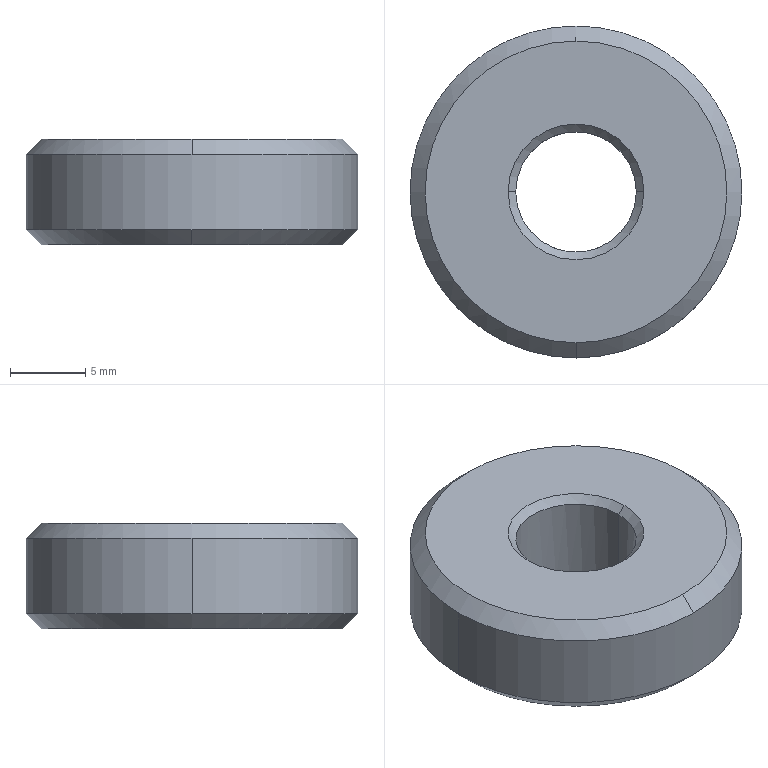Part | STEP file | MSBR-4_1_1_1_1 | 1 solid | 14 faces | box 22 x 22 x 7 mm | volume 2236 mm3 | cone 8 | cylinder 4 | plane 2 | commonest cylinder face diameters 8 x2 22 x2
STEP:
#1=CARTESIAN_POINT('',(0.,0.,0.));
#2=DIRECTION('',(0.,0.,1.));
#3=DIRECTION('',(1.,0.,0.));
#4=AXIS2_PLACEMENT_3D('',#1,#2,#3);
#5=CARTESIAN_POINT('',(-4.,0.,22.8));
#6=VERTEX_POINT('',#5);
#7=CARTESIAN_POINT('',(0.,4.,22.8));
#8=VERTEX_POINT('',#7);
#9=CARTESIAN_POINT('',(0.,0.,22.8));
#10=DIRECTION('',(0.,0.,-1.));
#11=DIRECTION('',(-1.,0.,0.));
#12=AXIS2_PLACEMENT_3D('',#9,#10,#11);
#13=CIRCLE('',#12,4.);
#14=EDGE_CURVE('',#6,#8,#13,.T.);
#15=ORIENTED_EDGE('',*,*,#14,.T.);
#16=CARTESIAN_POINT('',(0.,4.5,22.3));
#17=VERTEX_POINT('',#16);
#18=CARTESIAN_POINT('',(0.,4.5,22.3));
#19=DIRECTION('',(0.,-0.7071,0.7071));
#20=VECTOR('',#19,0.7071);
#21=LINE('',#18,#20);
#22=EDGE_CURVE('',#17,#8,#21,.T.);
#23=ORIENTED_EDGE('',*,*,#22,.F.);
#24=CARTESIAN_POINT('',(0.,-4.5,22.3));
#25=VERTEX_POINT('',#24);
#26=CARTESIAN_POINT('',(0.,0.,22.3));
#27=DIRECTION('',(0.,0.,-1.));
#28=DIRECTION('',(0.,-1.,0.));
#29=AXIS2_PLACEMENT_3D('',#26,#27,#28);
#30=CIRCLE('',#29,4.5);
#31=EDGE_CURVE('',#25,#17,#30,.T.);
#32=ORIENTED_EDGE('',*,*,#31,.F.);
#33=CARTESIAN_POINT('',(0.,-4.,22.8));
#34=VERTEX_POINT('',#33);
#35=CARTESIAN_POINT('',(0.,-4.,22.8));
#36=DIRECTION('',(0.,-0.7071,-0.7071));
#37=VECTOR('',#36,0.7071);
#38=LINE('',#35,#37);
#39=EDGE_CURVE('',#34,#25,#38,.T.);
#40=ORIENTED_EDGE('',*,*,#39,.F.);
#41=CARTESIAN_POINT('',(0.,0.,22.8));
#42=DIRECTION('',(0.,0.,-1.));
#43=DIRECTION('',(0.,-1.,0.));
#44=AXIS2_PLACEMENT_3D('',#41,#42,#43);
#45=CIRCLE('',#44,4.);
#46=EDGE_CURVE('',#34,#6,#45,.T.);
#47=ORIENTED_EDGE('',*,*,#46,.T.);
#48=EDGE_LOOP('',(#15,#23,#32,#40,#47));
#49=FACE_OUTER_BOUND('',#48,.F.);
#50=CARTESIAN_POINT('',(0.,0.,22.55));
#51=DIRECTION('',(0.,0.,-1.));
#52=DIRECTION('',(0.,1.,0.));
#53=AXIS2_PLACEMENT_3D('',#50,#51,#52);
#54=CONICAL_SURFACE('',#53,4.25,45.);
#55=ADVANCED_FACE('',(#49),#54,.F.);
#56=CARTESIAN_POINT('',(4.,0.,22.8));
#57=VERTEX_POINT('',#56);
#58=CARTESIAN_POINT('',(4.,0.,28.8));
#59=VERTEX_POINT('',#58);
#60=CARTESIAN_POINT('',(4.,0.,22.8));
#61=DIRECTION('',(0.000000023,0.,1.));
#62=VECTOR('',#61,6.);
#63=LINE('',#60,#62);
#64=EDGE_CURVE('',#57,#59,#63,.T.);
#65=ORIENTED_EDGE('',*,*,#64,.F.);
#66=CARTESIAN_POINT('',(0.,0.,22.8));
#67=DIRECTION('',(0.,0.,-1.));
#68=DIRECTION('',(0.,1.,0.));
#69=AXIS2_PLACEMENT_3D('',#66,#67,#68);
#70=CIRCLE('',#69,4.);
#71=EDGE_CURVE('',#8,#57,#70,.T.);
#72=ORIENTED_EDGE('',*,*,#71,.F.);
#73=ORIENTED_EDGE('',*,*,#14,.F.);
#74=CARTESIAN_POINT('',(-4.,0.,28.8));
#75=VERTEX_POINT('',#74);
#76=CARTESIAN_POINT('',(-4.,0.,28.8));
#77=DIRECTION('',(0.000000014,0.,-1.));
#78=VECTOR('',#77,6.);
#79=LINE('',#76,#78);
#80=EDGE_CURVE('',#75,#6,#79,.T.);
#81=ORIENTED_EDGE('',*,*,#80,.F.);
#82=CARTESIAN_POINT('',(0.,0.,28.8));
#83=DIRECTION('',(0.,-0.000000001,1.));
#84=DIRECTION('',(1.,0.,0.));
#85=AXIS2_PLACEMENT_3D('',#82,#83,#84);
#86=CIRCLE('',#85,4.);
#87=EDGE_CURVE('',#59,#75,#86,.T.);
#88=ORIENTED_EDGE('',*,*,#87,.F.);
#89=EDGE_LOOP('',(#65,#72,#73,#81,#88));
#90=FACE_OUTER_BOUND('',#89,.F.);
#91=CARTESIAN_POINT('',(0.,0.,28.92));
#92=DIRECTION('',(0.,0.,-1.));
#93=DIRECTION('',(-1.,0.,0.));
#94=AXIS2_PLACEMENT_3D('',#91,#92,#93);
#95=CYLINDRICAL_SURFACE('',#94,4.);
#96=ADVANCED_FACE('',(#90),#95,.F.);
#97=ORIENTED_EDGE('',*,*,#46,.F.);
#98=CARTESIAN_POINT('',(0.,0.,22.8));
#99=DIRECTION('',(0.,0.,-1.));
#100=DIRECTION('',(1.,0.,0.));
#101=AXIS2_PLACEMENT_3D('',#98,#99,#100);
#102=CIRCLE('',#101,4.);
#103=EDGE_CURVE('',#57,#34,#102,.T.);
#104=ORIENTED_EDGE('',*,*,#103,.F.);
#105=ORIENTED_EDGE('',*,*,#64,.T.);
#106=CARTESIAN_POINT('',(0.,0.,28.8));
#107=DIRECTION('',(0.,0.000000001,1.));
#108=DIRECTION('',(-1.,0.,0.));
#109=AXIS2_PLACEMENT_3D('',#106,#107,#108);
#110=CIRCLE('',#109,4.);
#111=EDGE_CURVE('',#75,#59,#110,.T.);
#112=ORIENTED_EDGE('',*,*,#111,.F.);
#113=ORIENTED_EDGE('',*,*,#80,.T.);
#114=EDGE_LOOP('',(#97,#104,#105,#112,#113));
#115=FACE_OUTER_BOUND('',#114,.F.);
#116=CARTESIAN_POINT('',(0.,0.,28.92));
#117=DIRECTION('',(0.,0.,-1.));
#118=DIRECTION('',(1.,0.,0.));
#119=AXIS2_PLACEMENT_3D('',#116,#117,#118);
#120=CYLINDRICAL_SURFACE('',#119,4.);
#121=ADVANCED_FACE('',(#115),#120,.F.);
#122=CARTESIAN_POINT('',(0.,0.,22.3));
#123=DIRECTION('',(0.,0.,-1.));
#124=DIRECTION('',(0.,1.,0.));
#125=AXIS2_PLACEMENT_3D('',#122,#123,#124);
#126=CIRCLE('',#125,4.5);
#127=EDGE_CURVE('',#17,#25,#126,.T.);
#128=ORIENTED_EDGE('',*,*,#127,.F.);
#129=ORIENTED_EDGE('',*,*,#22,.T.);
#130=ORIENTED_EDGE('',*,*,#71,.T.);
#131=ORIENTED_EDGE('',*,*,#103,.T.);
#132=ORIENTED_EDGE('',*,*,#39,.T.);
#133=EDGE_LOOP('',(#128,#129,#130,#131,#132));
#134=FACE_OUTER_BOUND('',#133,.F.);
#135=CARTESIAN_POINT('',(0.,0.,22.55));
#136=DIRECTION('',(0.,0.,-1.));
#137=DIRECTION('',(0.,-1.,0.));
#138=AXIS2_PLACEMENT_3D('',#135,#136,#137);
#139=CONICAL_SURFACE('',#138,4.25,45.);
#140=ADVANCED_FACE('',(#134),#139,.F.);
#141=CARTESIAN_POINT('',(0.,10.,22.3));
#142=VERTEX_POINT('',#141);
#143=CARTESIAN_POINT('',(0.,-10.,22.3));
#144=VERTEX_POINT('',#143);
#145=CARTESIAN_POINT('',(0.,0.,22.3));
#146=DIRECTION('',(0.,0.,1.));
#147=DIRECTION('',(0.,1.,0.));
#148=AXIS2_PLACEMENT_3D('',#145,#146,#147);
#149=CIRCLE('',#148,10.);
#150=EDGE_CURVE('',#142,#144,#149,.T.);
#151=ORIENTED_EDGE('',*,*,#150,.T.);
#152=CARTESIAN_POINT('',(0.,0.,22.3));
#153=DIRECTION('',(0.,0.,1.));
#154=DIRECTION('',(0.,-1.,0.));
#155=AXIS2_PLACEMENT_3D('',#152,#153,#154);
#156=CIRCLE('',#155,10.);
#157=EDGE_CURVE('',#144,#142,#156,.T.);
#158=ORIENTED_EDGE('',*,*,#157,.T.);
#159=EDGE_LOOP('',(#151,#158));
#160=FACE_OUTER_BOUND('',#159,.F.);
#161=ORIENTED_EDGE('',*,*,#31,.T.);
#162=ORIENTED_EDGE('',*,*,#127,.T.);
#163=EDGE_LOOP('',(#161,#162));
#164=FACE_BOUND('',#163,.F.);
#165=CARTESIAN_POINT('',(0.,0.,22.3));
#166=DIRECTION('',(0.,0.,1.));
#167=DIRECTION('',(-1.,0.,0.));
#168=AXIS2_PLACEMENT_3D('',#165,#166,#167);
#169=PLANE('',#168);
#170=ADVANCED_FACE('',(#160,#164),#169,.F.);
#171=CARTESIAN_POINT('',(0.,11.,23.3));
#172=VERTEX_POINT('',#171);
#173=CARTESIAN_POINT('',(0.,11.,23.3));
#174=DIRECTION('',(0.,-0.7071,-0.7071));
#175=VECTOR('',#174,1.414);
#176=LINE('',#173,#175);
#177=EDGE_CURVE('',#172,#142,#176,.T.);
#178=ORIENTED_EDGE('',*,*,#177,.F.);
#179=CARTESIAN_POINT('',(-11.,0.,23.3));
#180=VERTEX_POINT('',#179);
#181=CARTESIAN_POINT('',(0.,0.,23.3));
#182=DIRECTION('',(0.,0.,1.));
#183=DIRECTION('',(0.,1.,0.));
#184=AXIS2_PLACEMENT_3D('',#181,#182,#183);
#185=CIRCLE('',#184,11.);
#186=EDGE_CURVE('',#172,#180,#185,.T.);
#187=ORIENTED_EDGE('',*,*,#186,.T.);
#188=CARTESIAN_POINT('',(0.,-11.,23.3));
#189=VERTEX_POINT('',#188);
#190=CARTESIAN_POINT('',(0.,0.,23.3));
#191=DIRECTION('',(0.,0.,1.));
#192=DIRECTION('',(-1.,0.,0.));
#193=AXIS2_PLACEMENT_3D('',#190,#191,#192);
#194=CIRCLE('',#193,11.);
#195=EDGE_CURVE('',#180,#189,#194,.T.);
#196=ORIENTED_EDGE('',*,*,#195,.T.);
#197=CARTESIAN_POINT('',(0.,-10.,22.3));
#198=DIRECTION('',(0.,-0.7071,0.7071));
#199=VECTOR('',#198,1.414);
#200=LINE('',#197,#199);
#201=EDGE_CURVE('',#144,#189,#200,.T.);
#202=ORIENTED_EDGE('',*,*,#201,.F.);
#203=ORIENTED_EDGE('',*,*,#150,.F.);
#204=EDGE_LOOP('',(#178,#187,#196,#202,#203));
#205=FACE_OUTER_BOUND('',#204,.F.);
#206=CARTESIAN_POINT('',(0.,0.,22.8));
#207=DIRECTION('',(0.,0.,1.));
#208=DIRECTION('',(0.,-1.,0.));
#209=AXIS2_PLACEMENT_3D('',#206,#207,#208);
#210=CONICAL_SURFACE('',#209,10.5,45.);
#211=ADVANCED_FACE('',(#205),#210,.T.);
#212=ORIENTED_EDGE('',*,*,#157,.F.);
#213=ORIENTED_EDGE('',*,*,#201,.T.);
#214=CARTESIAN_POINT('',(11.,0.,23.3));
#215=VERTEX_POINT('',#214);
#216=CARTESIAN_POINT('',(0.,0.,23.3));
#217=DIRECTION('',(0.,0.,1.));
#218=DIRECTION('',(0.,-1.,0.));
#219=AXIS2_PLACEMENT_3D('',#216,#217,#218);
#220=CIRCLE('',#219,11.);
#221=EDGE_CURVE('',#189,#215,#220,.T.);
#222=ORIENTED_EDGE('',*,*,#221,.T.);
#223=CARTESIAN_POINT('',(0.,0.,23.3));
#224=DIRECTION('',(0.,0.,1.));
#225=DIRECTION('',(1.,0.,0.));
#226=AXIS2_PLACEMENT_3D('',#223,#224,#225);
#227=CIRCLE('',#226,11.);
#228=EDGE_CURVE('',#215,#172,#227,.T.);
#229=ORIENTED_EDGE('',*,*,#228,.T.);
#230=ORIENTED_EDGE('',*,*,#177,.T.);
#231=EDGE_LOOP('',(#212,#213,#222,#229,#230));
#232=FACE_OUTER_BOUND('',#231,.F.);
#233=CARTESIAN_POINT('',(0.,0.,22.8));
#234=DIRECTION('',(0.,0.,1.));
#235=DIRECTION('',(0.,1.,0.));
#236=AXIS2_PLACEMENT_3D('',#233,#234,#235);
#237=CONICAL_SURFACE('',#236,10.5,45.);
#238=ADVANCED_FACE('',(#232),#237,.T.);
#239=CARTESIAN_POINT('',(0.,-11.,28.3));
#240=VERTEX_POINT('',#239);
#241=CARTESIAN_POINT('',(-11.,0.,28.3));
#242=VERTEX_POINT('',#241);
#243=CARTESIAN_POINT('',(0.,0.,28.3));
#244=DIRECTION('',(0.000000001,0.,-1.));
#245=DIRECTION('',(0.,-1.,0.));
#246=AXIS2_PLACEMENT_3D('',#243,#244,#245);
#247=CIRCLE('',#246,11.);
#248=EDGE_CURVE('',#240,#242,#247,.T.);
#249=ORIENTED_EDGE('',*,*,#248,.F.);
#250=CARTESIAN_POINT('',(11.,0.,28.3));
#251=VERTEX_POINT('',#250);
#252=CARTESIAN_POINT('',(0.,0.,28.3));
#253=DIRECTION('',(-0.000000001,0.,-1.));
#254=DIRECTION('',(1.,0.,-0.000000001));
#255=AXIS2_PLACEMENT_3D('',#252,#253,#254);
#256=CIRCLE('',#255,11.);
#257=EDGE_CURVE('',#251,#240,#256,.T.);
#258=ORIENTED_EDGE('',*,*,#257,.F.);
#259=CARTESIAN_POINT('',(11.,0.,23.3));
#260=DIRECTION('',(-0.000000022,0.,1.));
#261=VECTOR('',#260,5.);
#262=LINE('',#259,#261);
#263=EDGE_CURVE('',#215,#251,#262,.T.);
#264=ORIENTED_EDGE('',*,*,#263,.F.);
#265=ORIENTED_EDGE('',*,*,#221,.F.);
#266=ORIENTED_EDGE('',*,*,#195,.F.);
#267=CARTESIAN_POINT('',(-11.,0.,28.3));
#268=DIRECTION('',(-0.000000011,0.,-1.));
#269=VECTOR('',#268,5.);
#270=LINE('',#267,#269);
#271=EDGE_CURVE('',#242,#180,#270,.T.);
#272=ORIENTED_EDGE('',*,*,#271,.F.);
#273=EDGE_LOOP('',(#249,#258,#264,#265,#266,#272));
#274=FACE_OUTER_BOUND('',#273,.F.);
#275=CARTESIAN_POINT('',(0.,0.,28.4));
#276=DIRECTION('',(0.,0.,-1.));
#277=DIRECTION('',(1.,0.,0.));
#278=AXIS2_PLACEMENT_3D('',#275,#276,#277);
#279=CYLINDRICAL_SURFACE('',#278,11.);
#280=ADVANCED_FACE('',(#274),#279,.T.);
#281=CARTESIAN_POINT('',(0.,-10.,29.3));
#282=VERTEX_POINT('',#281);
#283=CARTESIAN_POINT('',(0.,-11.,28.3));
#284=DIRECTION('',(0.,0.7071,0.7071));
#285=VECTOR('',#284,1.414);
#286=LINE('',#283,#285);
#287=EDGE_CURVE('',#240,#282,#286,.T.);
#288=ORIENTED_EDGE('',*,*,#287,.F.);
#289=ORIENTED_EDGE('',*,*,#248,.T.);
#290=CARTESIAN_POINT('',(0.,11.,28.3));
#291=VERTEX_POINT('',#290);
#292=CARTESIAN_POINT('',(0.,0.,28.3));
#293=DIRECTION('',(0.000000001,0.,-1.));
#294=DIRECTION('',(-1.,0.,-0.000000001));
#295=AXIS2_PLACEMENT_3D('',#292,#293,#294);
#296=CIRCLE('',#295,11.);
#297=EDGE_CURVE('',#242,#291,#296,.T.);
#298=ORIENTED_EDGE('',*,*,#297,.T.);
#299=CARTESIAN_POINT('',(0.,10.,29.3));
#300=VERTEX_POINT('',#299);
#301=CARTESIAN_POINT('',(0.,10.,29.3));
#302=DIRECTION('',(0.,0.7071,-0.7071));
#303=VECTOR('',#302,1.414);
#304=LINE('',#301,#303);
#305=EDGE_CURVE('',#300,#291,#304,.T.);
#306=ORIENTED_EDGE('',*,*,#305,.F.);
#307=CARTESIAN_POINT('',(-0.000000001,0.,29.3));
#308=DIRECTION('',(0.000000001,0.,-1.));
#309=DIRECTION('',(0.,-1.,0.));
#310=AXIS2_PLACEMENT_3D('',#307,#308,#309);
#311=CIRCLE('',#310,10.);
#312=EDGE_CURVE('',#282,#300,#311,.T.);
#313=ORIENTED_EDGE('',*,*,#312,.F.);
#314=EDGE_LOOP('',(#288,#289,#298,#306,#313));
#315=FACE_OUTER_BOUND('',#314,.F.);
#316=CARTESIAN_POINT('',(0.,0.,28.8));
#317=DIRECTION('',(0.000000001,0.,-1.));
#318=DIRECTION('',(0.,1.,0.));
#319=AXIS2_PLACEMENT_3D('',#316,#317,#318);
#320=CONICAL_SURFACE('',#319,10.5,45.);
#321=ADVANCED_FACE('',(#315),#320,.T.);
#322=CARTESIAN_POINT('',(0.000000001,0.,29.3));
#323=DIRECTION('',(-0.000000001,0.,-1.));
#324=DIRECTION('',(0.,1.,0.));
#325=AXIS2_PLACEMENT_3D('',#322,#323,#324);
#326=CIRCLE('',#325,10.);
#327=EDGE_CURVE('',#300,#282,#326,.T.);
#328=ORIENTED_EDGE('',*,*,#327,.F.);
#329=ORIENTED_EDGE('',*,*,#305,.T.);
#330=CARTESIAN_POINT('',(0.,0.,28.3));
#331=DIRECTION('',(-0.000000001,0.,-1.));
#332=DIRECTION('',(0.,1.,0.));
#333=AXIS2_PLACEMENT_3D('',#330,#331,#332);
#334=CIRCLE('',#333,11.);
#335=EDGE_CURVE('',#291,#251,#334,.T.);
#336=ORIENTED_EDGE('',*,*,#335,.T.);
#337=ORIENTED_EDGE('',*,*,#257,.T.);
#338=ORIENTED_EDGE('',*,*,#287,.T.);
#339=EDGE_LOOP('',(#328,#329,#336,#337,#338));
#340=FACE_OUTER_BOUND('',#339,.F.);
#341=CARTESIAN_POINT('',(0.,0.,28.8));
#342=DIRECTION('',(-0.000000001,0.,-1.));
#343=DIRECTION('',(0.,-1.,0.));
#344=AXIS2_PLACEMENT_3D('',#341,#342,#343);
#345=CONICAL_SURFACE('',#344,10.5,45.);
#346=ADVANCED_FACE('',(#340),#345,.T.);
#347=ORIENTED_EDGE('',*,*,#312,.T.);
#348=ORIENTED_EDGE('',*,*,#327,.T.);
#349=EDGE_LOOP('',(#347,#348));
#350=FACE_OUTER_BOUND('',#349,.F.);
#351=CARTESIAN_POINT('',(-4.5,0.,29.3));
#352=VERTEX_POINT('',#351);
#353=CARTESIAN_POINT('',(4.5,0.,29.3));
#354=VERTEX_POINT('',#353);
#355=CARTESIAN_POINT('',(0.,0.,29.3));
#356=DIRECTION('',(0.,0.000000001,1.));
#357=DIRECTION('',(-1.,0.,0.));
#358=AXIS2_PLACEMENT_3D('',#355,#356,#357);
#359=CIRCLE('',#358,4.5);
#360=EDGE_CURVE('',#352,#354,#359,.T.);
#361=ORIENTED_EDGE('',*,*,#360,.T.);
#362=CARTESIAN_POINT('',(0.,0.,29.3));
#363=DIRECTION('',(0.,-0.000000001,1.));
#364=DIRECTION('',(1.,0.,0.));
#365=AXIS2_PLACEMENT_3D('',#362,#363,#364);
#366=CIRCLE('',#365,4.5);
#367=EDGE_CURVE('',#354,#352,#366,.T.);
#368=ORIENTED_EDGE('',*,*,#367,.T.);
#369=EDGE_LOOP('',(#361,#368));
#370=FACE_BOUND('',#369,.F.);
#371=CARTESIAN_POINT('',(0.,0.,29.3));
#372=DIRECTION('',(0.,0.,1.));
#373=DIRECTION('',(-1.,0.,0.));
#374=AXIS2_PLACEMENT_3D('',#371,#372,#373);
#375=PLANE('',#374);
#376=ADVANCED_FACE('',(#350,#370),#375,.T.);
#377=ORIENTED_EDGE('',*,*,#360,.F.);
#378=CARTESIAN_POINT('',(-4.,0.,28.8));
#379=DIRECTION('',(-0.7071,0.,0.7071));
#380=VECTOR('',#379,0.7071);
#381=LINE('',#378,#380);
#382=EDGE_CURVE('',#75,#352,#381,.T.);
#383=ORIENTED_EDGE('',*,*,#382,.F.);
#384=ORIENTED_EDGE('',*,*,#111,.T.);
#385=CARTESIAN_POINT('',(4.5,0.,29.3));
#386=DIRECTION('',(-0.7071,0.,-0.7071));
#387=VECTOR('',#386,0.7071);
#388=LINE('',#385,#387);
#389=EDGE_CURVE('',#354,#59,#388,.T.);
#390=ORIENTED_EDGE('',*,*,#389,.F.);
#391=EDGE_LOOP('',(#377,#383,#384,#390));
#392=FACE_OUTER_BOUND('',#391,.F.);
#393=CARTESIAN_POINT('',(0.,0.,29.05));
#394=DIRECTION('',(0.,0.000000001,1.));
#395=DIRECTION('',(1.,0.,0.));
#396=AXIS2_PLACEMENT_3D('',#393,#394,#395);
#397=CONICAL_SURFACE('',#396,4.25,45.);
#398=ADVANCED_FACE('',(#392),#397,.F.);
#399=ORIENTED_EDGE('',*,*,#382,.T.);
#400=ORIENTED_EDGE('',*,*,#367,.F.);
#401=ORIENTED_EDGE('',*,*,#389,.T.);
#402=ORIENTED_EDGE('',*,*,#87,.T.);
#403=EDGE_LOOP('',(#399,#400,#401,#402));
#404=FACE_OUTER_BOUND('',#403,.F.);
#405=CARTESIAN_POINT('',(0.,0.,29.05));
#406=DIRECTION('',(0.,-0.000000001,1.));
#407=DIRECTION('',(-1.,0.,0.));
#408=AXIS2_PLACEMENT_3D('',#405,#406,#407);
#409=CONICAL_SURFACE('',#408,4.25,45.);
#410=ADVANCED_FACE('',(#404),#409,.F.);
#411=ORIENTED_EDGE('',*,*,#271,.T.);
#412=ORIENTED_EDGE('',*,*,#186,.F.);
#413=ORIENTED_EDGE('',*,*,#228,.F.);
#414=ORIENTED_EDGE('',*,*,#263,.T.);
#415=ORIENTED_EDGE('',*,*,#335,.F.);
#416=ORIENTED_EDGE('',*,*,#297,.F.);
#417=EDGE_LOOP('',(#411,#412,#413,#414,#415,#416));
#418=FACE_OUTER_BOUND('',#417,.F.);
#419=CARTESIAN_POINT('',(0.,0.,28.4));
#420=DIRECTION('',(0.,0.,-1.));
#421=DIRECTION('',(-1.,0.,0.));
#422=AXIS2_PLACEMENT_3D('',#419,#420,#421);
#423=CYLINDRICAL_SURFACE('',#422,11.);
#424=ADVANCED_FACE('',(#418),#423,.T.);
#425=CLOSED_SHELL('',(#55,#96,#121,#140,#170,#211,#238,#280,#321,#346,#376,#398,#410,#424));
#426=MANIFOLD_SOLID_BREP('',#425);
#427=(LENGTH_UNIT()NAMED_UNIT(*)SI_UNIT(.MILLI.,.METRE.));
#428=UNCERTAINTY_MEASURE_WITH_UNIT(LENGTH_MEASURE(0.003189),#427,'','');
#429=(NAMED_UNIT(*)PLANE_ANGLE_UNIT()SI_UNIT($,.RADIAN.));
#430=PLANE_ANGLE_MEASURE_WITH_UNIT(PLANE_ANGLE_MEASURE(0.01745),#429);
#431=(CONVERSION_BASED_UNIT('DEGREE',#430)NAMED_UNIT(*)PLANE_ANGLE_UNIT());
#432=(NAMED_UNIT(*)SI_UNIT($,.STERADIAN.)SOLID_ANGLE_UNIT());
#433=(GEOMETRIC_REPRESENTATION_CONTEXT(3)GLOBAL_UNCERTAINTY_ASSIGNED_CONTEXT((#428))GLOBAL_UNIT_ASSIGNED_CONTEXT((#427,#431,#432))REPRESENTATION_CONTEXT('',''));
#434=ADVANCED_BREP_SHAPE_REPRESENTATION('',(#4,#426),#433);